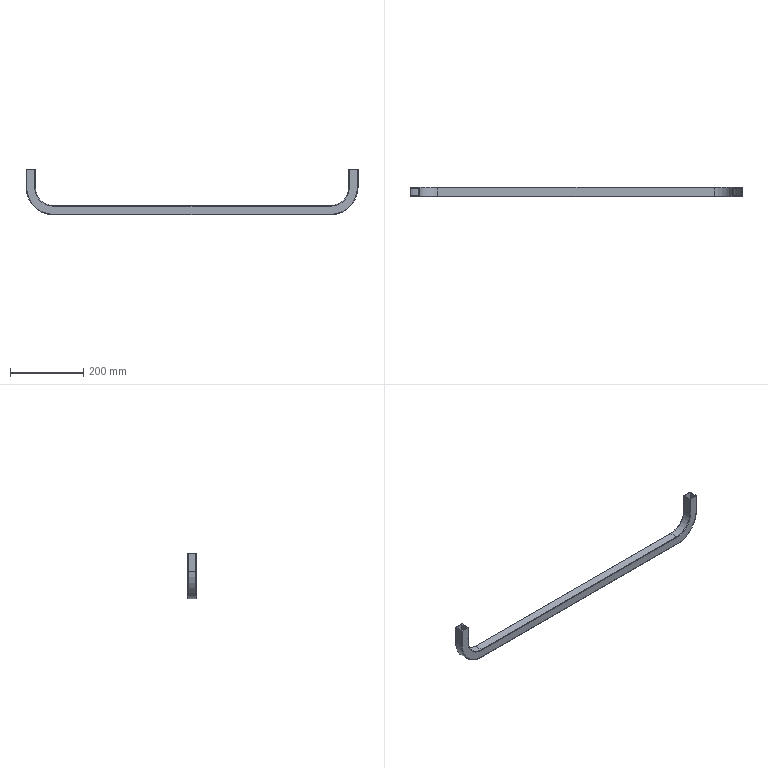Part | NX | features BREP 1 | 1 solid | 46 faces | box 908.05 x 25.4 x 125.476 mm | volume 193275 mm3 | cylinder 20 | plane 18 | torus 8 | commonest cylinder face diameters 3.175 x12 101.6 x2 105.562 x2 148.438 x2 152.4 x2
STEP:
#1=CARTESIAN_POINT('',(454.025,11.113,0.));
#2=VERTEX_POINT('',#1);
#3=CARTESIAN_POINT('',(452.438,12.7,0.));
#4=VERTEX_POINT('',#3);
#5=CARTESIAN_POINT('',(452.438,11.113,0.));
#6=DIRECTION('',(0.,0.,1.));
#7=DIRECTION('',(1.,0.,0.));
#8=AXIS2_PLACEMENT_3D('',#5,#6,#7);
#9=CIRCLE('',#8,1.588);
#10=EDGE_CURVE('',#2,#4,#9,.T.);
#11=ORIENTED_EDGE('',*,*,#10,.T.);
#12=CARTESIAN_POINT('',(430.212,12.7,0.));
#13=VERTEX_POINT('',#12);
#14=CARTESIAN_POINT('',(430.212,12.7,0.));
#15=DIRECTION('',(1.,0.,0.));
#16=VECTOR('',#15,1000.);
#17=LINE('',#14,#16);
#18=EDGE_CURVE('',#13,#4,#17,.T.);
#19=ORIENTED_EDGE('',*,*,#18,.F.);
#20=CARTESIAN_POINT('',(428.625,11.113,0.));
#21=VERTEX_POINT('',#20);
#22=CARTESIAN_POINT('',(430.212,11.113,0.));
#23=DIRECTION('',(0.,0.,1.));
#24=DIRECTION('',(0.,1.,0.));
#25=AXIS2_PLACEMENT_3D('',#22,#23,#24);
#26=CIRCLE('',#25,1.587);
#27=EDGE_CURVE('',#13,#21,#26,.T.);
#28=ORIENTED_EDGE('',*,*,#27,.T.);
#29=CARTESIAN_POINT('',(428.625,-11.113,0.));
#30=VERTEX_POINT('',#29);
#31=CARTESIAN_POINT('',(428.625,-11.113,0.));
#32=DIRECTION('',(0.,1.,0.));
#33=VECTOR('',#32,1000.);
#34=LINE('',#31,#33);
#35=EDGE_CURVE('',#30,#21,#34,.T.);
#36=ORIENTED_EDGE('',*,*,#35,.F.);
#37=CARTESIAN_POINT('',(430.212,-12.7,0.));
#38=VERTEX_POINT('',#37);
#39=CARTESIAN_POINT('',(430.212,-11.113,0.));
#40=DIRECTION('',(0.,0.,1.));
#41=DIRECTION('',(-1.,0.,0.));
#42=AXIS2_PLACEMENT_3D('',#39,#40,#41);
#43=CIRCLE('',#42,1.588);
#44=EDGE_CURVE('',#30,#38,#43,.T.);
#45=ORIENTED_EDGE('',*,*,#44,.T.);
#46=CARTESIAN_POINT('',(452.438,-12.7,0.));
#47=VERTEX_POINT('',#46);
#48=CARTESIAN_POINT('',(452.438,-12.7,0.));
#49=DIRECTION('',(-1.,0.,0.));
#50=VECTOR('',#49,1000.);
#51=LINE('',#48,#50);
#52=EDGE_CURVE('',#47,#38,#51,.T.);
#53=ORIENTED_EDGE('',*,*,#52,.F.);
#54=CARTESIAN_POINT('',(454.025,-11.113,0.));
#55=VERTEX_POINT('',#54);
#56=CARTESIAN_POINT('',(452.438,-11.113,0.));
#57=DIRECTION('',(0.,0.,1.));
#58=DIRECTION('',(0.,-1.,0.));
#59=AXIS2_PLACEMENT_3D('',#56,#57,#58);
#60=CIRCLE('',#59,1.587);
#61=EDGE_CURVE('',#47,#55,#60,.T.);
#62=ORIENTED_EDGE('',*,*,#61,.T.);
#63=CARTESIAN_POINT('',(454.025,11.113,0.));
#64=DIRECTION('',(0.,-1.,0.));
#65=VECTOR('',#64,1000.);
#66=LINE('',#63,#65);
#67=EDGE_CURVE('',#2,#55,#66,.T.);
#68=ORIENTED_EDGE('',*,*,#67,.F.);
#69=EDGE_LOOP('',(#11,#19,#28,#36,#45,#53,#62,#68));
#70=FACE_BOUND('',#69,.T.);
#71=CARTESIAN_POINT('',(452.044,-10.719,0.));
#72=VERTEX_POINT('',#71);
#73=CARTESIAN_POINT('',(452.044,10.719,0.));
#74=VERTEX_POINT('',#73);
#75=CARTESIAN_POINT('',(452.044,-10.719,0.));
#76=DIRECTION('',(0.,1.,0.));
#77=VECTOR('',#76,1000.);
#78=LINE('',#75,#77);
#79=EDGE_CURVE('',#72,#74,#78,.T.);
#80=ORIENTED_EDGE('',*,*,#79,.F.);
#81=CARTESIAN_POINT('',(430.606,-10.719,0.));
#82=VERTEX_POINT('',#81);
#83=CARTESIAN_POINT('',(430.606,-10.719,0.));
#84=DIRECTION('',(1.,0.,0.));
#85=VECTOR('',#84,1000.);
#86=LINE('',#83,#85);
#87=EDGE_CURVE('',#82,#72,#86,.T.);
#88=ORIENTED_EDGE('',*,*,#87,.F.);
#89=CARTESIAN_POINT('',(430.606,10.719,0.));
#90=VERTEX_POINT('',#89);
#91=CARTESIAN_POINT('',(430.606,10.719,0.));
#92=DIRECTION('',(0.,-1.,0.));
#93=VECTOR('',#92,1000.);
#94=LINE('',#91,#93);
#95=EDGE_CURVE('',#90,#82,#94,.T.);
#96=ORIENTED_EDGE('',*,*,#95,.F.);
#97=CARTESIAN_POINT('',(452.044,10.719,0.));
#98=DIRECTION('',(-1.,0.,0.));
#99=VECTOR('',#98,1000.);
#100=LINE('',#97,#99);
#101=EDGE_CURVE('',#74,#90,#100,.T.);
#102=ORIENTED_EDGE('',*,*,#101,.F.);
#103=EDGE_LOOP('',(#80,#88,#96,#102));
#104=FACE_BOUND('',#103,.T.);
#105=CARTESIAN_POINT('',(441.325,0.,0.));
#106=DIRECTION('',(0.,0.,-1.));
#107=DIRECTION('',(0.,-1.,0.));
#108=AXIS2_PLACEMENT_3D('',#105,#106,#107);
#109=PLANE('',#108);
#110=ADVANCED_FACE('',(#70,#104),#109,.F.);
#111=CARTESIAN_POINT('',(430.606,10.719,-49.276));
#112=VERTEX_POINT('',#111);
#113=CARTESIAN_POINT('',(430.606,10.719,0.));
#114=DIRECTION('',(0.,0.,-1.));
#115=VECTOR('',#114,1000.);
#116=LINE('',#113,#115);
#117=EDGE_CURVE('',#90,#112,#116,.T.);
#118=ORIENTED_EDGE('',*,*,#117,.T.);
#119=CARTESIAN_POINT('',(377.825,10.719,-102.057));
#120=VERTEX_POINT('',#119);
#121=CARTESIAN_POINT('',(377.825,10.719,-49.276));
#122=DIRECTION('',(0.,1.,0.));
#123=DIRECTION('',(1.,0.,0.));
#124=AXIS2_PLACEMENT_3D('',#121,#122,#123);
#125=CIRCLE('',#124,52.781);
#126=EDGE_CURVE('',#112,#120,#125,.T.);
#127=ORIENTED_EDGE('',*,*,#126,.T.);
#128=CARTESIAN_POINT('',(-377.825,10.719,-102.057));
#129=VERTEX_POINT('',#128);
#130=CARTESIAN_POINT('',(377.825,10.719,-102.057));
#131=DIRECTION('',(-1.,0.,0.));
#132=VECTOR('',#131,1000.);
#133=LINE('',#130,#132);
#134=EDGE_CURVE('',#120,#129,#133,.T.);
#135=ORIENTED_EDGE('',*,*,#134,.T.);
#136=CARTESIAN_POINT('',(-430.606,10.719,-49.276));
#137=VERTEX_POINT('',#136);
#138=CARTESIAN_POINT('',(-377.825,10.719,-49.276));
#139=DIRECTION('',(0.,1.,0.));
#140=DIRECTION('',(0.,0.,-1.));
#141=AXIS2_PLACEMENT_3D('',#138,#139,#140);
#142=CIRCLE('',#141,52.781);
#143=EDGE_CURVE('',#129,#137,#142,.T.);
#144=ORIENTED_EDGE('',*,*,#143,.T.);
#145=CARTESIAN_POINT('',(-430.606,10.719,0.));
#146=VERTEX_POINT('',#145);
#147=CARTESIAN_POINT('',(-430.606,10.719,-49.276));
#148=DIRECTION('',(0.,0.,1.));
#149=VECTOR('',#148,1000.);
#150=LINE('',#147,#149);
#151=EDGE_CURVE('',#137,#146,#150,.T.);
#152=ORIENTED_EDGE('',*,*,#151,.T.);
#153=CARTESIAN_POINT('',(-452.044,10.719,0.));
#154=VERTEX_POINT('',#153);
#155=CARTESIAN_POINT('',(-452.044,10.719,0.));
#156=DIRECTION('',(1.,0.,0.));
#157=VECTOR('',#156,1000.);
#158=LINE('',#155,#157);
#159=EDGE_CURVE('',#154,#146,#158,.T.);
#160=ORIENTED_EDGE('',*,*,#159,.F.);
#161=CARTESIAN_POINT('',(-452.044,10.719,-49.276));
#162=VERTEX_POINT('',#161);
#163=CARTESIAN_POINT('',(-452.044,10.719,-49.276));
#164=DIRECTION('',(0.,0.,1.));
#165=VECTOR('',#164,1000.);
#166=LINE('',#163,#165);
#167=EDGE_CURVE('',#162,#154,#166,.T.);
#168=ORIENTED_EDGE('',*,*,#167,.F.);
#169=CARTESIAN_POINT('',(-377.825,10.719,-123.495));
#170=VERTEX_POINT('',#169);
#171=CARTESIAN_POINT('',(-377.825,10.719,-49.276));
#172=DIRECTION('',(0.,1.,0.));
#173=DIRECTION('',(0.,0.,-1.));
#174=AXIS2_PLACEMENT_3D('',#171,#172,#173);
#175=CIRCLE('',#174,74.219);
#176=EDGE_CURVE('',#170,#162,#175,.T.);
#177=ORIENTED_EDGE('',*,*,#176,.F.);
#178=CARTESIAN_POINT('',(377.825,10.719,-123.495));
#179=VERTEX_POINT('',#178);
#180=CARTESIAN_POINT('',(377.825,10.719,-123.495));
#181=DIRECTION('',(-1.,0.,0.));
#182=VECTOR('',#181,1000.);
#183=LINE('',#180,#182);
#184=EDGE_CURVE('',#179,#170,#183,.T.);
#185=ORIENTED_EDGE('',*,*,#184,.F.);
#186=CARTESIAN_POINT('',(452.044,10.719,-49.276));
#187=VERTEX_POINT('',#186);
#188=CARTESIAN_POINT('',(377.825,10.719,-49.276));
#189=DIRECTION('',(0.,1.,0.));
#190=DIRECTION('',(1.,0.,0.));
#191=AXIS2_PLACEMENT_3D('',#188,#189,#190);
#192=CIRCLE('',#191,74.219);
#193=EDGE_CURVE('',#187,#179,#192,.T.);
#194=ORIENTED_EDGE('',*,*,#193,.F.);
#195=CARTESIAN_POINT('',(452.044,10.719,0.));
#196=DIRECTION('',(0.,0.,-1.));
#197=VECTOR('',#196,1000.);
#198=LINE('',#195,#197);
#199=EDGE_CURVE('',#74,#187,#198,.T.);
#200=ORIENTED_EDGE('',*,*,#199,.F.);
#201=ORIENTED_EDGE('',*,*,#101,.T.);
#202=EDGE_LOOP('',(#118,#127,#135,#144,#152,#160,#168,#177,#185,#194,#200,#201));
#203=FACE_BOUND('',#202,.T.);
#204=CARTESIAN_POINT('',(452.044,10.719,0.));
#205=DIRECTION('',(0.,-1.,0.));
#206=DIRECTION('',(0.,0.,-1.));
#207=AXIS2_PLACEMENT_3D('',#204,#205,#206);
#208=PLANE('',#207);
#209=ADVANCED_FACE('',(#203),#208,.T.);
#210=ORIENTED_EDGE('',*,*,#199,.T.);
#211=CARTESIAN_POINT('',(452.044,-10.719,-49.276));
#212=VERTEX_POINT('',#211);
#213=CARTESIAN_POINT('',(452.044,-10.719,-49.276));
#214=DIRECTION('',(0.,1.,0.));
#215=VECTOR('',#214,1000.);
#216=LINE('',#213,#215);
#217=EDGE_CURVE('',#212,#187,#216,.T.);
#218=ORIENTED_EDGE('',*,*,#217,.F.);
#219=CARTESIAN_POINT('',(452.044,-10.719,0.));
#220=DIRECTION('',(0.,0.,-1.));
#221=VECTOR('',#220,1000.);
#222=LINE('',#219,#221);
#223=EDGE_CURVE('',#72,#212,#222,.T.);
#224=ORIENTED_EDGE('',*,*,#223,.F.);
#225=ORIENTED_EDGE('',*,*,#79,.T.);
#226=EDGE_LOOP('',(#210,#218,#224,#225));
#227=FACE_BOUND('',#226,.T.);
#228=CARTESIAN_POINT('',(452.044,-10.719,0.));
#229=DIRECTION('',(-1.,0.,0.));
#230=DIRECTION('',(0.,0.,1.));
#231=AXIS2_PLACEMENT_3D('',#228,#229,#230);
#232=PLANE('',#231);
#233=ADVANCED_FACE('',(#227),#232,.T.);
#234=ORIENTED_EDGE('',*,*,#223,.T.);
#235=CARTESIAN_POINT('',(377.825,-10.719,-123.495));
#236=VERTEX_POINT('',#235);
#237=CARTESIAN_POINT('',(377.825,-10.719,-49.276));
#238=DIRECTION('',(0.,1.,0.));
#239=DIRECTION('',(1.,0.,0.));
#240=AXIS2_PLACEMENT_3D('',#237,#238,#239);
#241=CIRCLE('',#240,74.219);
#242=EDGE_CURVE('',#212,#236,#241,.T.);
#243=ORIENTED_EDGE('',*,*,#242,.T.);
#244=CARTESIAN_POINT('',(-377.825,-10.719,-123.495));
#245=VERTEX_POINT('',#244);
#246=CARTESIAN_POINT('',(377.825,-10.719,-123.495));
#247=DIRECTION('',(-1.,0.,0.));
#248=VECTOR('',#247,1000.);
#249=LINE('',#246,#248);
#250=EDGE_CURVE('',#236,#245,#249,.T.);
#251=ORIENTED_EDGE('',*,*,#250,.T.);
#252=CARTESIAN_POINT('',(-452.044,-10.719,-49.276));
#253=VERTEX_POINT('',#252);
#254=CARTESIAN_POINT('',(-377.825,-10.719,-49.276));
#255=DIRECTION('',(0.,1.,0.));
#256=DIRECTION('',(0.,0.,-1.));
#257=AXIS2_PLACEMENT_3D('',#254,#255,#256);
#258=CIRCLE('',#257,74.219);
#259=EDGE_CURVE('',#245,#253,#258,.T.);
#260=ORIENTED_EDGE('',*,*,#259,.T.);
#261=CARTESIAN_POINT('',(-452.044,-10.719,0.));
#262=VERTEX_POINT('',#261);
#263=CARTESIAN_POINT('',(-452.044,-10.719,-49.276));
#264=DIRECTION('',(0.,0.,1.));
#265=VECTOR('',#264,1000.);
#266=LINE('',#263,#265);
#267=EDGE_CURVE('',#253,#262,#266,.T.);
#268=ORIENTED_EDGE('',*,*,#267,.T.);
#269=CARTESIAN_POINT('',(-430.606,-10.719,0.));
#270=VERTEX_POINT('',#269);
#271=CARTESIAN_POINT('',(-430.606,-10.719,0.));
#272=DIRECTION('',(-1.,0.,0.));
#273=VECTOR('',#272,1000.);
#274=LINE('',#271,#273);
#275=EDGE_CURVE('',#270,#262,#274,.T.);
#276=ORIENTED_EDGE('',*,*,#275,.F.);
#277=CARTESIAN_POINT('',(-430.606,-10.719,-49.276));
#278=VERTEX_POINT('',#277);
#279=CARTESIAN_POINT('',(-430.606,-10.719,-49.276));
#280=DIRECTION('',(0.,0.,1.));
#281=VECTOR('',#280,1000.);
#282=LINE('',#279,#281);
#283=EDGE_CURVE('',#278,#270,#282,.T.);
#284=ORIENTED_EDGE('',*,*,#283,.F.);
#285=CARTESIAN_POINT('',(-377.825,-10.719,-102.057));
#286=VERTEX_POINT('',#285);
#287=CARTESIAN_POINT('',(-377.825,-10.719,-49.276));
#288=DIRECTION('',(0.,1.,0.));
#289=DIRECTION('',(0.,0.,-1.));
#290=AXIS2_PLACEMENT_3D('',#287,#288,#289);
#291=CIRCLE('',#290,52.781);
#292=EDGE_CURVE('',#286,#278,#291,.T.);
#293=ORIENTED_EDGE('',*,*,#292,.F.);
#294=CARTESIAN_POINT('',(377.825,-10.719,-102.057));
#295=VERTEX_POINT('',#294);
#296=CARTESIAN_POINT('',(377.825,-10.719,-102.057));
#297=DIRECTION('',(-1.,0.,0.));
#298=VECTOR('',#297,1000.);
#299=LINE('',#296,#298);
#300=EDGE_CURVE('',#295,#286,#299,.T.);
#301=ORIENTED_EDGE('',*,*,#300,.F.);
#302=CARTESIAN_POINT('',(430.606,-10.719,-49.276));
#303=VERTEX_POINT('',#302);
#304=CARTESIAN_POINT('',(377.825,-10.719,-49.276));
#305=DIRECTION('',(0.,1.,0.));
#306=DIRECTION('',(1.,0.,0.));
#307=AXIS2_PLACEMENT_3D('',#304,#305,#306);
#308=CIRCLE('',#307,52.781);
#309=EDGE_CURVE('',#303,#295,#308,.T.);
#310=ORIENTED_EDGE('',*,*,#309,.F.);
#311=CARTESIAN_POINT('',(430.606,-10.719,0.));
#312=DIRECTION('',(0.,0.,-1.));
#313=VECTOR('',#312,1000.);
#314=LINE('',#311,#313);
#315=EDGE_CURVE('',#82,#303,#314,.T.);
#316=ORIENTED_EDGE('',*,*,#315,.F.);
#317=ORIENTED_EDGE('',*,*,#87,.T.);
#318=EDGE_LOOP('',(#234,#243,#251,#260,#268,#276,#284,#293,#301,#310,#316,#317));
#319=FACE_BOUND('',#318,.T.);
#320=CARTESIAN_POINT('',(430.606,-10.719,0.));
#321=DIRECTION('',(0.,1.,0.));
#322=DIRECTION('',(1.,0.,0.));
#323=AXIS2_PLACEMENT_3D('',#320,#321,#322);
#324=PLANE('',#323);
#325=ADVANCED_FACE('',(#319),#324,.T.);
#326=ORIENTED_EDGE('',*,*,#315,.T.);
#327=CARTESIAN_POINT('',(430.606,10.719,-49.276));
#328=DIRECTION('',(0.,-1.,0.));
#329=VECTOR('',#328,1000.);
#330=LINE('',#327,#329);
#331=EDGE_CURVE('',#112,#303,#330,.T.);
#332=ORIENTED_EDGE('',*,*,#331,.F.);
#333=ORIENTED_EDGE('',*,*,#117,.F.);
#334=ORIENTED_EDGE('',*,*,#95,.T.);
#335=EDGE_LOOP('',(#326,#332,#333,#334));
#336=FACE_BOUND('',#335,.T.);
#337=CARTESIAN_POINT('',(430.606,10.719,0.));
#338=DIRECTION('',(1.,0.,0.));
#339=DIRECTION('',(0.,1.,0.));
#340=AXIS2_PLACEMENT_3D('',#337,#338,#339);
#341=PLANE('',#340);
#342=ADVANCED_FACE('',(#336),#341,.T.);
#343=ORIENTED_EDGE('',*,*,#309,.T.);
#344=CARTESIAN_POINT('',(377.825,10.719,-102.057));
#345=DIRECTION('',(0.,-1.,0.));
#346=VECTOR('',#345,1000.);
#347=LINE('',#344,#346);
#348=EDGE_CURVE('',#120,#295,#347,.T.);
#349=ORIENTED_EDGE('',*,*,#348,.F.);
#350=ORIENTED_EDGE('',*,*,#126,.F.);
#351=ORIENTED_EDGE('',*,*,#331,.T.);
#352=EDGE_LOOP('',(#343,#349,#350,#351));
#353=FACE_BOUND('',#352,.T.);
#354=CARTESIAN_POINT('',(377.825,-25.4,-49.276));
#355=DIRECTION('',(0.,1.,0.));
#356=DIRECTION('',(-1.,0.,0.));
#357=AXIS2_PLACEMENT_3D('',#354,#355,#356);
#358=CYLINDRICAL_SURFACE('',#357,52.781);
#359=ADVANCED_FACE('',(#353),#358,.T.);
#360=ORIENTED_EDGE('',*,*,#300,.T.);
#361=CARTESIAN_POINT('',(-377.825,10.719,-102.057));
#362=DIRECTION('',(0.,-1.,0.));
#363=VECTOR('',#362,1000.);
#364=LINE('',#361,#363);
#365=EDGE_CURVE('',#129,#286,#364,.T.);
#366=ORIENTED_EDGE('',*,*,#365,.F.);
#367=ORIENTED_EDGE('',*,*,#134,.F.);
#368=ORIENTED_EDGE('',*,*,#348,.T.);
#369=EDGE_LOOP('',(#360,#366,#367,#368));
#370=FACE_BOUND('',#369,.T.);
#371=CARTESIAN_POINT('',(377.825,10.719,-102.057));
#372=DIRECTION('',(0.,0.,-1.));
#373=DIRECTION('',(0.,-1.,0.));
#374=AXIS2_PLACEMENT_3D('',#371,#372,#373);
#375=PLANE('',#374);
#376=ADVANCED_FACE('',(#370),#375,.T.);
#377=ORIENTED_EDGE('',*,*,#292,.T.);
#378=CARTESIAN_POINT('',(-430.606,10.719,-49.276));
#379=DIRECTION('',(0.,-1.,0.));
#380=VECTOR('',#379,1000.);
#381=LINE('',#378,#380);
#382=EDGE_CURVE('',#137,#278,#381,.T.);
#383=ORIENTED_EDGE('',*,*,#382,.F.);
#384=ORIENTED_EDGE('',*,*,#143,.F.);
#385=ORIENTED_EDGE('',*,*,#365,.T.);
#386=EDGE_LOOP('',(#377,#383,#384,#385));
#387=FACE_BOUND('',#386,.T.);
#388=CARTESIAN_POINT('',(-377.825,-25.4,-49.276));
#389=DIRECTION('',(0.,1.,0.));
#390=DIRECTION('',(0.,0.,1.));
#391=AXIS2_PLACEMENT_3D('',#388,#389,#390);
#392=CYLINDRICAL_SURFACE('',#391,52.781);
#393=ADVANCED_FACE('',(#387),#392,.T.);
#394=ORIENTED_EDGE('',*,*,#283,.T.);
#395=CARTESIAN_POINT('',(-430.606,10.719,0.));
#396=DIRECTION('',(0.,-1.,0.));
#397=VECTOR('',#396,1000.);
#398=LINE('',#395,#397);
#399=EDGE_CURVE('',#146,#270,#398,.T.);
#400=ORIENTED_EDGE('',*,*,#399,.F.);
#401=ORIENTED_EDGE('',*,*,#151,.F.);
#402=ORIENTED_EDGE('',*,*,#382,.T.);
#403=EDGE_LOOP('',(#394,#400,#401,#402));
#404=FACE_BOUND('',#403,.T.);
#405=CARTESIAN_POINT('',(-430.606,10.719,-49.276));
#406=DIRECTION('',(-1.,0.,0.));
#407=DIRECTION('',(0.,0.,1.));
#408=AXIS2_PLACEMENT_3D('',#405,#406,#407);
#409=PLANE('',#408);
#410=ADVANCED_FACE('',(#404),#409,.T.);
#411=CARTESIAN_POINT('',(-454.025,-11.113,0.));
#412=VERTEX_POINT('',#411);
#413=CARTESIAN_POINT('',(-452.438,-12.7,0.));
#414=VERTEX_POINT('',#413);
#415=CARTESIAN_POINT('',(-452.438,-11.113,0.));
#416=DIRECTION('',(0.,0.,1.));
#417=DIRECTION('',(-1.,0.,0.));
#418=AXIS2_PLACEMENT_3D('',#415,#416,#417);
#419=CIRCLE('',#418,1.588);
#420=EDGE_CURVE('',#412,#414,#419,.T.);
#421=ORIENTED_EDGE('',*,*,#420,.T.);
#422=CARTESIAN_POINT('',(-430.212,-12.7,0.));
#423=VERTEX_POINT('',#422);
#424=CARTESIAN_POINT('',(-452.438,-12.7,0.));
#425=DIRECTION('',(1.,0.,0.));
#426=VECTOR('',#425,1000.);
#427=LINE('',#424,#426);
#428=EDGE_CURVE('',#414,#423,#427,.T.);
#429=ORIENTED_EDGE('',*,*,#428,.T.);
#430=CARTESIAN_POINT('',(-428.625,-11.113,0.));
#431=VERTEX_POINT('',#430);
#432=CARTESIAN_POINT('',(-430.212,-11.113,0.));
#433=DIRECTION('',(0.,0.,1.));
#434=DIRECTION('',(0.,-1.,0.));
#435=AXIS2_PLACEMENT_3D('',#432,#433,#434);
#436=CIRCLE('',#435,1.587);
#437=EDGE_CURVE('',#423,#431,#436,.T.);
#438=ORIENTED_EDGE('',*,*,#437,.T.);
#439=CARTESIAN_POINT('',(-428.625,11.113,0.));
#440=VERTEX_POINT('',#439);
#441=CARTESIAN_POINT('',(-428.625,-11.113,0.));
#442=DIRECTION('',(0.,1.,0.));
#443=VECTOR('',#442,1000.);
#444=LINE('',#441,#443);
#445=EDGE_CURVE('',#431,#440,#444,.T.);
#446=ORIENTED_EDGE('',*,*,#445,.T.);
#447=CARTESIAN_POINT('',(-430.212,12.7,0.));
#448=VERTEX_POINT('',#447);
#449=CARTESIAN_POINT('',(-430.212,11.113,0.));
#450=DIRECTION('',(0.,0.,1.));
#451=DIRECTION('',(1.,0.,0.));
#452=AXIS2_PLACEMENT_3D('',#449,#450,#451);
#453=CIRCLE('',#452,1.588);
#454=EDGE_CURVE('',#440,#448,#453,.T.);
#455=ORIENTED_EDGE('',*,*,#454,.T.);
#456=CARTESIAN_POINT('',(-452.438,12.7,0.));
#457=VERTEX_POINT('',#456);
#458=CARTESIAN_POINT('',(-430.212,12.7,0.));
#459=DIRECTION('',(-1.,0.,0.));
#460=VECTOR('',#459,1000.);
#461=LINE('',#458,#460);
#462=EDGE_CURVE('',#448,#457,#461,.T.);
#463=ORIENTED_EDGE('',*,*,#462,.T.);
#464=CARTESIAN_POINT('',(-454.025,11.113,0.));
#465=VERTEX_POINT('',#464);
#466=CARTESIAN_POINT('',(-452.438,11.113,0.));
#467=DIRECTION('',(0.,0.,1.));
#468=DIRECTION('',(0.,1.,0.));
#469=AXIS2_PLACEMENT_3D('',#466,#467,#468);
#470=CIRCLE('',#469,1.587);
#471=EDGE_CURVE('',#457,#465,#470,.T.);
#472=ORIENTED_EDGE('',*,*,#471,.T.);
#473=CARTESIAN_POINT('',(-454.025,11.113,0.));
#474=DIRECTION('',(0.,-1.,0.));
#475=VECTOR('',#474,1000.);
#476=LINE('',#473,#475);
#477=EDGE_CURVE('',#465,#412,#476,.T.);
#478=ORIENTED_EDGE('',*,*,#477,.T.);
#479=EDGE_LOOP('',(#421,#429,#438,#446,#455,#463,#472,#478));
#480=FACE_BOUND('',#479,.T.);
#481=ORIENTED_EDGE('',*,*,#399,.T.);
#482=ORIENTED_EDGE('',*,*,#275,.T.);
#483=CARTESIAN_POINT('',(-452.044,-10.719,0.));
#484=DIRECTION('',(0.,1.,0.));
#485=VECTOR('',#484,1000.);
#486=LINE('',#483,#485);
#487=EDGE_CURVE('',#262,#154,#486,.T.);
#488=ORIENTED_EDGE('',*,*,#487,.T.);
#489=ORIENTED_EDGE('',*,*,#159,.T.);
#490=EDGE_LOOP('',(#481,#482,#488,#489));
#491=FACE_BOUND('',#490,.T.);
#492=CARTESIAN_POINT('',(-441.325,0.,0.));
#493=DIRECTION('',(0.,0.,1.));
#494=DIRECTION('',(1.,0.,0.));
#495=AXIS2_PLACEMENT_3D('',#492,#493,#494);
#496=PLANE('',#495);
#497=ADVANCED_FACE('',(#480,#491),#496,.T.);
#498=ORIENTED_EDGE('',*,*,#167,.T.);
#499=ORIENTED_EDGE('',*,*,#487,.F.);
#500=ORIENTED_EDGE('',*,*,#267,.F.);
#501=CARTESIAN_POINT('',(-452.044,-10.719,-49.276));
#502=DIRECTION('',(0.,1.,0.));
#503=VECTOR('',#502,1000.);
#504=LINE('',#501,#503);
#505=EDGE_CURVE('',#253,#162,#504,.T.);
#506=ORIENTED_EDGE('',*,*,#505,.T.);
#507=EDGE_LOOP('',(#498,#499,#500,#506));
#508=FACE_BOUND('',#507,.T.);
#509=CARTESIAN_POINT('',(-452.044,-10.719,-49.276));
#510=DIRECTION('',(1.,0.,0.));
#511=DIRECTION('',(0.,1.,0.));
#512=AXIS2_PLACEMENT_3D('',#509,#510,#511);
#513=PLANE('',#512);
#514=ADVANCED_FACE('',(#508),#513,.T.);
#515=ORIENTED_EDGE('',*,*,#176,.T.);
#516=ORIENTED_EDGE('',*,*,#505,.F.);
#517=ORIENTED_EDGE('',*,*,#259,.F.);
#518=CARTESIAN_POINT('',(-377.825,-10.719,-123.495));
#519=DIRECTION('',(0.,1.,0.));
#520=VECTOR('',#519,1000.);
#521=LINE('',#518,#520);
#522=EDGE_CURVE('',#245,#170,#521,.T.);
#523=ORIENTED_EDGE('',*,*,#522,.T.);
#524=EDGE_LOOP('',(#515,#516,#517,#523));
#525=FACE_BOUND('',#524,.T.);
#526=CARTESIAN_POINT('',(-377.825,-25.4,-49.276));
#527=DIRECTION('',(0.,1.,0.));
#528=DIRECTION('',(0.,0.,1.));
#529=AXIS2_PLACEMENT_3D('',#526,#527,#528);
#530=CYLINDRICAL_SURFACE('',#529,74.219);
#531=ADVANCED_FACE('',(#525),#530,.F.);
#532=ORIENTED_EDGE('',*,*,#184,.T.);
#533=ORIENTED_EDGE('',*,*,#522,.F.);
#534=ORIENTED_EDGE('',*,*,#250,.F.);
#535=CARTESIAN_POINT('',(377.825,-10.719,-123.495));
#536=DIRECTION('',(0.,1.,0.));
#537=VECTOR('',#536,1000.);
#538=LINE('',#535,#537);
#539=EDGE_CURVE('',#236,#179,#538,.T.);
#540=ORIENTED_EDGE('',*,*,#539,.T.);
#541=EDGE_LOOP('',(#532,#533,#534,#540));
#542=FACE_BOUND('',#541,.T.);
#543=CARTESIAN_POINT('',(377.825,-10.719,-123.495));
#544=DIRECTION('',(0.,0.,1.));
#545=DIRECTION('',(1.,0.,0.));
#546=AXIS2_PLACEMENT_3D('',#543,#544,#545);
#547=PLANE('',#546);
#548=ADVANCED_FACE('',(#542),#547,.T.);
#549=ORIENTED_EDGE('',*,*,#193,.T.);
#550=ORIENTED_EDGE('',*,*,#539,.F.);
#551=ORIENTED_EDGE('',*,*,#242,.F.);
#552=ORIENTED_EDGE('',*,*,#217,.T.);
#553=EDGE_LOOP('',(#549,#550,#551,#552));
#554=FACE_BOUND('',#553,.T.);
#555=CARTESIAN_POINT('',(377.825,-25.4,-49.276));
#556=DIRECTION('',(0.,1.,0.));
#557=DIRECTION('',(-1.,0.,0.));
#558=AXIS2_PLACEMENT_3D('',#555,#556,#557);
#559=CYLINDRICAL_SURFACE('',#558,74.219);
#560=ADVANCED_FACE('',(#554),#559,.F.);
#561=CARTESIAN_POINT('',(-454.025,-11.113,-49.276));
#562=VERTEX_POINT('',#561);
#563=CARTESIAN_POINT('',(-454.025,-11.113,0.));
#564=DIRECTION('',(0.,0.,-1.));
#565=VECTOR('',#564,1000.);
#566=LINE('',#563,#565);
#567=EDGE_CURVE('',#412,#562,#566,.T.);
#568=ORIENTED_EDGE('',*,*,#567,.F.);
#569=ORIENTED_EDGE('',*,*,#477,.F.);
#570=CARTESIAN_POINT('',(-454.025,11.113,-49.276));
#571=VERTEX_POINT('',#570);
#572=CARTESIAN_POINT('',(-454.025,11.113,0.));
#573=DIRECTION('',(0.,0.,-1.));
#574=VECTOR('',#573,1000.);
#575=LINE('',#572,#574);
#576=EDGE_CURVE('',#465,#571,#575,.T.);
#577=ORIENTED_EDGE('',*,*,#576,.T.);
#578=CARTESIAN_POINT('',(-454.025,11.113,-49.276));
#579=DIRECTION('',(0.,-1.,0.));
#580=VECTOR('',#579,1000.);
#581=LINE('',#578,#580);
#582=EDGE_CURVE('',#571,#562,#581,.T.);
#583=ORIENTED_EDGE('',*,*,#582,.T.);
#584=EDGE_LOOP('',(#568,#569,#577,#583));
#585=FACE_BOUND('',#584,.T.);
#586=CARTESIAN_POINT('',(-454.025,12.7,-49.276));
#587=DIRECTION('',(-1.,0.,0.));
#588=DIRECTION('',(0.,0.,1.));
#589=AXIS2_PLACEMENT_3D('',#586,#587,#588);
#590=PLANE('',#589);
#591=ADVANCED_FACE('',(#585),#590,.T.);
#592=CARTESIAN_POINT('',(-377.825,11.113,-125.476));
#593=VERTEX_POINT('',#592);
#594=CARTESIAN_POINT('',(-377.825,11.113,-49.276));
#595=DIRECTION('',(0.,-1.,0.));
#596=DIRECTION('',(-1.,0.,0.));
#597=AXIS2_PLACEMENT_3D('',#594,#595,#596);
#598=CIRCLE('',#597,76.2);
#599=EDGE_CURVE('',#571,#593,#598,.T.);
#600=ORIENTED_EDGE('',*,*,#599,.T.);
#601=CARTESIAN_POINT('',(-377.825,-11.113,-125.476));
#602=VERTEX_POINT('',#601);
#603=CARTESIAN_POINT('',(-377.825,11.113,-125.476));
#604=DIRECTION('',(0.,-1.,0.));
#605=VECTOR('',#604,1000.);
#606=LINE('',#603,#605);
#607=EDGE_CURVE('',#593,#602,#606,.T.);
#608=ORIENTED_EDGE('',*,*,#607,.T.);
#609=CARTESIAN_POINT('',(-377.825,-11.113,-49.276));
#610=DIRECTION('',(0.,-1.,0.));
#611=DIRECTION('',(-1.,0.,0.));
#612=AXIS2_PLACEMENT_3D('',#609,#610,#611);
#613=CIRCLE('',#612,76.2);
#614=EDGE_CURVE('',#562,#602,#613,.T.);
#615=ORIENTED_EDGE('',*,*,#614,.F.);
#616=ORIENTED_EDGE('',*,*,#582,.F.);
#617=EDGE_LOOP('',(#600,#608,#615,#616));
#618=FACE_BOUND('',#617,.T.);
#619=CARTESIAN_POINT('',(-377.825,-25.4,-49.276));
#620=DIRECTION('',(0.,1.,0.));
#621=DIRECTION('',(0.,0.,1.));
#622=AXIS2_PLACEMENT_3D('',#619,#620,#621);
#623=CYLINDRICAL_SURFACE('',#622,76.2);
#624=ADVANCED_FACE('',(#618),#623,.T.);
#625=CARTESIAN_POINT('',(-452.438,-12.7,-49.276));
#626=VERTEX_POINT('',#625);
#627=CARTESIAN_POINT('',(-452.438,-11.113,-49.276));
#628=DIRECTION('',(0.,0.,-1.));
#629=DIRECTION('',(0.,-1.,0.));
#630=AXIS2_PLACEMENT_3D('',#627,#628,#629);
#631=CIRCLE('',#630,1.587);
#632=EDGE_CURVE('',#626,#562,#631,.T.);
#633=ORIENTED_EDGE('',*,*,#632,.T.);
#634=ORIENTED_EDGE('',*,*,#614,.T.);
#635=CARTESIAN_POINT('',(-377.825,-12.7,-123.888));
#636=VERTEX_POINT('',#635);
#637=CARTESIAN_POINT('',(-377.825,-11.113,-123.888));
#638=DIRECTION('',(1.,0.,0.));
#639=DIRECTION('',(0.,-1.,0.));
#640=AXIS2_PLACEMENT_3D('',#637,#638,#639);
#641=CIRCLE('',#640,1.587);
#642=EDGE_CURVE('',#636,#602,#641,.T.);
#643=ORIENTED_EDGE('',*,*,#642,.F.);
#644=CARTESIAN_POINT('',(-377.825,-12.7,-49.276));
#645=DIRECTION('',(0.,-1.,0.));
#646=DIRECTION('',(-1.,0.,0.));
#647=AXIS2_PLACEMENT_3D('',#644,#645,#646);
#648=CIRCLE('',#647,74.613);
#649=EDGE_CURVE('',#626,#636,#648,.T.);
#650=ORIENTED_EDGE('',*,*,#649,.F.);
#651=EDGE_LOOP('',(#633,#634,#643,#650));
#652=FACE_BOUND('',#651,.T.);
#653=CARTESIAN_POINT('',(-377.825,-11.113,-49.276));
#654=DIRECTION('',(0.,1.,0.));
#655=DIRECTION('',(-0.9997,0.,0.02628));
#656=AXIS2_PLACEMENT_3D('',#653,#654,#655);
#657=TOROIDAL_SURFACE('',#656,74.612,1.587);
#658=ADVANCED_FACE('',(#652),#657,.T.);
#659=CARTESIAN_POINT('',(430.212,-12.7,-49.276));
#660=VERTEX_POINT('',#659);
#661=CARTESIAN_POINT('',(430.212,-12.7,-49.276));
#662=DIRECTION('',(0.,0.,1.));
#663=VECTOR('',#662,1000.);
#664=LINE('',#661,#663);
#665=EDGE_CURVE('',#660,#38,#664,.T.);
#666=ORIENTED_EDGE('',*,*,#665,.F.);
#667=CARTESIAN_POINT('',(377.825,-12.7,-101.664));
#668=VERTEX_POINT('',#667);
#669=CARTESIAN_POINT('',(377.825,-12.7,-49.276));
#670=DIRECTION('',(0.,-1.,0.));
#671=DIRECTION('',(0.,0.,-1.));
#672=AXIS2_PLACEMENT_3D('',#669,#670,#671);
#673=CIRCLE('',#672,52.388);
#674=EDGE_CURVE('',#668,#660,#673,.T.);
#675=ORIENTED_EDGE('',*,*,#674,.F.);
#676=CARTESIAN_POINT('',(-377.825,-12.7,-101.663));
#677=VERTEX_POINT('',#676);
#678=CARTESIAN_POINT('',(-377.825,-12.7,-101.663));
#679=DIRECTION('',(1.,0.,0.));
#680=VECTOR('',#679,1000.);
#681=LINE('',#678,#680);
#682=EDGE_CURVE('',#677,#668,#681,.T.);
#683=ORIENTED_EDGE('',*,*,#682,.F.);
#684=CARTESIAN_POINT('',(-430.213,-12.7,-49.276));
#685=VERTEX_POINT('',#684);
#686=CARTESIAN_POINT('',(-377.825,-12.7,-49.276));
#687=DIRECTION('',(0.,-1.,0.));
#688=DIRECTION('',(-1.,0.,0.));
#689=AXIS2_PLACEMENT_3D('',#686,#687,#688);
#690=CIRCLE('',#689,52.388);
#691=EDGE_CURVE('',#685,#677,#690,.T.);
#692=ORIENTED_EDGE('',*,*,#691,.F.);
#693=CARTESIAN_POINT('',(-430.212,-12.7,0.));
#694=DIRECTION('',(0.,0.,-1.));
#695=VECTOR('',#694,1000.);
#696=LINE('',#693,#695);
#697=EDGE_CURVE('',#423,#685,#696,.T.);
#698=ORIENTED_EDGE('',*,*,#697,.F.);
#699=ORIENTED_EDGE('',*,*,#428,.F.);
#700=CARTESIAN_POINT('',(-452.438,-12.7,0.));
#701=DIRECTION('',(0.,0.,-1.));
#702=VECTOR('',#701,1000.);
#703=LINE('',#700,#702);
#704=EDGE_CURVE('',#414,#626,#703,.T.);
#705=ORIENTED_EDGE('',*,*,#704,.T.);
#706=ORIENTED_EDGE('',*,*,#649,.T.);
#707=CARTESIAN_POINT('',(377.825,-12.7,-123.889));
#708=VERTEX_POINT('',#707);
#709=CARTESIAN_POINT('',(-377.825,-12.7,-123.888));
#710=DIRECTION('',(1.,0.,0.));
#711=VECTOR('',#710,1000.);
#712=LINE('',#709,#711);
#713=EDGE_CURVE('',#636,#708,#712,.T.);
#714=ORIENTED_EDGE('',*,*,#713,.T.);
#715=CARTESIAN_POINT('',(452.438,-12.7,-49.276));
#716=VERTEX_POINT('',#715);
#717=CARTESIAN_POINT('',(377.825,-12.7,-49.276));
#718=DIRECTION('',(0.,-1.,0.));
#719=DIRECTION('',(0.,0.,-1.));
#720=AXIS2_PLACEMENT_3D('',#717,#718,#719);
#721=CIRCLE('',#720,74.613);
#722=EDGE_CURVE('',#708,#716,#721,.T.);
#723=ORIENTED_EDGE('',*,*,#722,.T.);
#724=CARTESIAN_POINT('',(452.438,-12.7,-49.276));
#725=DIRECTION('',(0.,0.,1.));
#726=VECTOR('',#725,1000.);
#727=LINE('',#724,#726);
#728=EDGE_CURVE('',#716,#47,#727,.T.);
#729=ORIENTED_EDGE('',*,*,#728,.T.);
#730=ORIENTED_EDGE('',*,*,#52,.T.);
#731=EDGE_LOOP('',(#666,#675,#683,#692,#698,#699,#705,#706,#714,#723,#729,#730));
#732=FACE_BOUND('',#731,.T.);
#733=CARTESIAN_POINT('',(454.025,-12.7,0.));
#734=DIRECTION('',(0.,-1.,0.));
#735=DIRECTION('',(0.,0.,-1.));
#736=AXIS2_PLACEMENT_3D('',#733,#734,#735);
#737=PLANE('',#736);
#738=ADVANCED_FACE('',(#732),#737,.T.);
#739=CARTESIAN_POINT('',(454.025,-11.113,-49.276));
#740=VERTEX_POINT('',#739);
#741=CARTESIAN_POINT('',(452.438,-11.113,-49.276));
#742=DIRECTION('',(0.,0.,1.));
#743=DIRECTION('',(0.,-1.,0.));
#744=AXIS2_PLACEMENT_3D('',#741,#742,#743);
#745=CIRCLE('',#744,1.587);
#746=EDGE_CURVE('',#716,#740,#745,.T.);
#747=ORIENTED_EDGE('',*,*,#746,.T.);
#748=CARTESIAN_POINT('',(454.025,-11.113,-49.276));
#749=DIRECTION('',(0.,0.,1.));
#750=VECTOR('',#749,1000.);
#751=LINE('',#748,#750);
#752=EDGE_CURVE('',#740,#55,#751,.T.);
#753=ORIENTED_EDGE('',*,*,#752,.T.);
#754=ORIENTED_EDGE('',*,*,#61,.F.);
#755=ORIENTED_EDGE('',*,*,#728,.F.);
#756=EDGE_LOOP('',(#747,#753,#754,#755));
#757=FACE_BOUND('',#756,.T.);
#758=CARTESIAN_POINT('',(452.438,-11.113,-51.392));
#759=DIRECTION('',(0.,0.,1.));
#760=DIRECTION('',(0.,-1.,0.));
#761=AXIS2_PLACEMENT_3D('',#758,#759,#760);
#762=CYLINDRICAL_SURFACE('',#761,1.587);
#763=ADVANCED_FACE('',(#757),#762,.T.);
#764=ORIENTED_EDGE('',*,*,#752,.F.);
#765=CARTESIAN_POINT('',(454.025,11.113,-49.276));
#766=VERTEX_POINT('',#765);
#767=CARTESIAN_POINT('',(454.025,11.113,-49.276));
#768=DIRECTION('',(0.,-1.,0.));
#769=VECTOR('',#768,1000.);
#770=LINE('',#767,#769);
#771=EDGE_CURVE('',#766,#740,#770,.T.);
#772=ORIENTED_EDGE('',*,*,#771,.F.);
#773=CARTESIAN_POINT('',(454.025,11.113,-49.276));
#774=DIRECTION('',(0.,0.,1.));
#775=VECTOR('',#774,1000.);
#776=LINE('',#773,#775);
#777=EDGE_CURVE('',#766,#2,#776,.T.);
#778=ORIENTED_EDGE('',*,*,#777,.T.);
#779=ORIENTED_EDGE('',*,*,#67,.T.);
#780=EDGE_LOOP('',(#764,#772,#778,#779));
#781=FACE_BOUND('',#780,.T.);
#782=CARTESIAN_POINT('',(454.025,12.7,0.));
#783=DIRECTION('',(1.,0.,0.));
#784=DIRECTION('',(0.,1.,0.));
#785=AXIS2_PLACEMENT_3D('',#782,#783,#784);
#786=PLANE('',#785);
#787=ADVANCED_FACE('',(#781),#786,.T.);
#788=CARTESIAN_POINT('',(452.438,12.7,-49.276));
#789=VERTEX_POINT('',#788);
#790=CARTESIAN_POINT('',(452.438,11.113,-49.276));
#791=DIRECTION('',(0.,0.,1.));
#792=DIRECTION('',(1.,0.,0.));
#793=AXIS2_PLACEMENT_3D('',#790,#791,#792);
#794=CIRCLE('',#793,1.588);
#795=EDGE_CURVE('',#766,#789,#794,.T.);
#796=ORIENTED_EDGE('',*,*,#795,.T.);
#797=CARTESIAN_POINT('',(452.438,12.7,-49.276));
#798=DIRECTION('',(0.,0.,1.));
#799=VECTOR('',#798,1000.);
#800=LINE('',#797,#799);
#801=EDGE_CURVE('',#789,#4,#800,.T.);
#802=ORIENTED_EDGE('',*,*,#801,.T.);
#803=ORIENTED_EDGE('',*,*,#10,.F.);
#804=ORIENTED_EDGE('',*,*,#777,.F.);
#805=EDGE_LOOP('',(#796,#802,#803,#804));
#806=FACE_BOUND('',#805,.T.);
#807=CARTESIAN_POINT('',(452.438,11.113,-50.711));
#808=DIRECTION('',(0.,0.,1.));
#809=DIRECTION('',(1.,0.,0.));
#810=AXIS2_PLACEMENT_3D('',#807,#808,#809);
#811=CYLINDRICAL_SURFACE('',#810,1.588);
#812=ADVANCED_FACE('',(#806),#811,.T.);
#813=ORIENTED_EDGE('',*,*,#801,.F.);
#814=CARTESIAN_POINT('',(377.825,12.7,-123.888));
#815=VERTEX_POINT('',#814);
#816=CARTESIAN_POINT('',(377.825,12.7,-49.276));
#817=DIRECTION('',(0.,-1.,0.));
#818=DIRECTION('',(0.,0.,-1.));
#819=AXIS2_PLACEMENT_3D('',#816,#817,#818);
#820=CIRCLE('',#819,74.612);
#821=EDGE_CURVE('',#815,#789,#820,.T.);
#822=ORIENTED_EDGE('',*,*,#821,.F.);
#823=CARTESIAN_POINT('',(-377.825,12.7,-123.888));
#824=VERTEX_POINT('',#823);
#825=CARTESIAN_POINT('',(-377.825,12.7,-123.888));
#826=DIRECTION('',(1.,0.,0.));
#827=VECTOR('',#826,1000.);
#828=LINE('',#825,#827);
#829=EDGE_CURVE('',#824,#815,#828,.T.);
#830=ORIENTED_EDGE('',*,*,#829,.F.);
#831=CARTESIAN_POINT('',(-452.438,12.7,-49.276));
#832=VERTEX_POINT('',#831);
#833=CARTESIAN_POINT('',(-377.825,12.7,-49.276));
#834=DIRECTION('',(0.,-1.,0.));
#835=DIRECTION('',(-1.,0.,0.));
#836=AXIS2_PLACEMENT_3D('',#833,#834,#835);
#837=CIRCLE('',#836,74.613);
#838=EDGE_CURVE('',#832,#824,#837,.T.);
#839=ORIENTED_EDGE('',*,*,#838,.F.);
#840=CARTESIAN_POINT('',(-452.438,12.7,0.));
#841=DIRECTION('',(0.,0.,-1.));
#842=VECTOR('',#841,1000.);
#843=LINE('',#840,#842);
#844=EDGE_CURVE('',#457,#832,#843,.T.);
#845=ORIENTED_EDGE('',*,*,#844,.F.);
#846=ORIENTED_EDGE('',*,*,#462,.F.);
#847=CARTESIAN_POINT('',(-430.212,12.7,-49.276));
#848=VERTEX_POINT('',#847);
#849=CARTESIAN_POINT('',(-430.212,12.7,0.));
#850=DIRECTION('',(0.,0.,-1.));
#851=VECTOR('',#850,1000.);
#852=LINE('',#849,#851);
#853=EDGE_CURVE('',#448,#848,#852,.T.);
#854=ORIENTED_EDGE('',*,*,#853,.T.);
#855=CARTESIAN_POINT('',(-377.825,12.7,-101.663));
#856=VERTEX_POINT('',#855);
#857=CARTESIAN_POINT('',(-377.825,12.7,-49.276));
#858=DIRECTION('',(0.,-1.,0.));
#859=DIRECTION('',(-1.,0.,0.));
#860=AXIS2_PLACEMENT_3D('',#857,#858,#859);
#861=CIRCLE('',#860,52.387);
#862=EDGE_CURVE('',#848,#856,#861,.T.);
#863=ORIENTED_EDGE('',*,*,#862,.T.);
#864=CARTESIAN_POINT('',(377.825,12.7,-101.663));
#865=VERTEX_POINT('',#864);
#866=CARTESIAN_POINT('',(-377.825,12.7,-101.663));
#867=DIRECTION('',(1.,0.,0.));
#868=VECTOR('',#867,1000.);
#869=LINE('',#866,#868);
#870=EDGE_CURVE('',#856,#865,#869,.T.);
#871=ORIENTED_EDGE('',*,*,#870,.T.);
#872=CARTESIAN_POINT('',(430.212,12.7,-49.276));
#873=VERTEX_POINT('',#872);
#874=CARTESIAN_POINT('',(377.825,12.7,-49.276));
#875=DIRECTION('',(0.,-1.,0.));
#876=DIRECTION('',(0.,0.,-1.));
#877=AXIS2_PLACEMENT_3D('',#874,#875,#876);
#878=CIRCLE('',#877,52.387);
#879=EDGE_CURVE('',#865,#873,#878,.T.);
#880=ORIENTED_EDGE('',*,*,#879,.T.);
#881=CARTESIAN_POINT('',(430.212,12.7,-49.276));
#882=DIRECTION('',(0.,0.,1.));
#883=VECTOR('',#882,1000.);
#884=LINE('',#881,#883);
#885=EDGE_CURVE('',#873,#13,#884,.T.);
#886=ORIENTED_EDGE('',*,*,#885,.T.);
#887=ORIENTED_EDGE('',*,*,#18,.T.);
#888=EDGE_LOOP('',(#813,#822,#830,#839,#845,#846,#854,#863,#871,#880,#886,#887));
#889=FACE_BOUND('',#888,.T.);
#890=CARTESIAN_POINT('',(428.625,12.7,0.));
#891=DIRECTION('',(0.,1.,0.));
#892=DIRECTION('',(1.,0.,0.));
#893=AXIS2_PLACEMENT_3D('',#890,#891,#892);
#894=PLANE('',#893);
#895=ADVANCED_FACE('',(#889),#894,.T.);
#896=CARTESIAN_POINT('',(428.625,11.113,-49.276));
#897=VERTEX_POINT('',#896);
#898=CARTESIAN_POINT('',(430.212,11.113,-49.276));
#899=DIRECTION('',(0.,0.,1.));
#900=DIRECTION('',(0.,1.,0.));
#901=AXIS2_PLACEMENT_3D('',#898,#899,#900);
#902=CIRCLE('',#901,1.587);
#903=EDGE_CURVE('',#873,#897,#902,.T.);
#904=ORIENTED_EDGE('',*,*,#903,.T.);
#905=CARTESIAN_POINT('',(428.625,11.113,-49.276));
#906=DIRECTION('',(0.,0.,1.));
#907=VECTOR('',#906,1000.);
#908=LINE('',#905,#907);
#909=EDGE_CURVE('',#897,#21,#908,.T.);
#910=ORIENTED_EDGE('',*,*,#909,.T.);
#911=ORIENTED_EDGE('',*,*,#27,.F.);
#912=ORIENTED_EDGE('',*,*,#885,.F.);
#913=EDGE_LOOP('',(#904,#910,#911,#912));
#914=FACE_BOUND('',#913,.T.);
#915=CARTESIAN_POINT('',(430.212,11.113,-51.392));
#916=DIRECTION('',(0.,0.,1.));
#917=DIRECTION('',(0.,1.,0.));
#918=AXIS2_PLACEMENT_3D('',#915,#916,#917);
#919=CYLINDRICAL_SURFACE('',#918,1.587);
#920=ADVANCED_FACE('',(#914),#919,.T.);
#921=ORIENTED_EDGE('',*,*,#909,.F.);
#922=CARTESIAN_POINT('',(428.625,-11.113,-49.276));
#923=VERTEX_POINT('',#922);
#924=CARTESIAN_POINT('',(428.625,-11.113,-49.276));
#925=DIRECTION('',(0.,1.,0.));
#926=VECTOR('',#925,1000.);
#927=LINE('',#924,#926);
#928=EDGE_CURVE('',#923,#897,#927,.T.);
#929=ORIENTED_EDGE('',*,*,#928,.F.);
#930=CARTESIAN_POINT('',(428.625,-11.113,-49.276));
#931=DIRECTION('',(0.,0.,1.));
#932=VECTOR('',#931,1000.);
#933=LINE('',#930,#932);
#934=EDGE_CURVE('',#923,#30,#933,.T.);
#935=ORIENTED_EDGE('',*,*,#934,.T.);
#936=ORIENTED_EDGE('',*,*,#35,.T.);
#937=EDGE_LOOP('',(#921,#929,#935,#936));
#938=FACE_BOUND('',#937,.T.);
#939=CARTESIAN_POINT('',(428.625,-12.7,0.));
#940=DIRECTION('',(-1.,0.,0.));
#941=DIRECTION('',(0.,0.,1.));
#942=AXIS2_PLACEMENT_3D('',#939,#940,#941);
#943=PLANE('',#942);
#944=ADVANCED_FACE('',(#938),#943,.T.);
#945=CARTESIAN_POINT('',(430.212,-11.113,-49.276));
#946=DIRECTION('',(0.,0.,1.));
#947=DIRECTION('',(-1.,0.,0.));
#948=AXIS2_PLACEMENT_3D('',#945,#946,#947);
#949=CIRCLE('',#948,1.588);
#950=EDGE_CURVE('',#923,#660,#949,.T.);
#951=ORIENTED_EDGE('',*,*,#950,.T.);
#952=ORIENTED_EDGE('',*,*,#665,.T.);
#953=ORIENTED_EDGE('',*,*,#44,.F.);
#954=ORIENTED_EDGE('',*,*,#934,.F.);
#955=EDGE_LOOP('',(#951,#952,#953,#954));
#956=FACE_BOUND('',#955,.T.);
#957=CARTESIAN_POINT('',(430.212,-11.113,-50.711));
#958=DIRECTION('',(0.,0.,1.));
#959=DIRECTION('',(-1.,0.,0.));
#960=AXIS2_PLACEMENT_3D('',#957,#958,#959);
#961=CYLINDRICAL_SURFACE('',#960,1.588);
#962=ADVANCED_FACE('',(#956),#961,.T.);
#963=CARTESIAN_POINT('',(377.825,-11.113,-100.076));
#964=VERTEX_POINT('',#963);
#965=CARTESIAN_POINT('',(377.825,-11.113,-101.663));
#966=DIRECTION('',(1.,0.,0.));
#967=DIRECTION('',(0.,0.,1.));
#968=AXIS2_PLACEMENT_3D('',#965,#966,#967);
#969=CIRCLE('',#968,1.588);
#970=EDGE_CURVE('',#964,#668,#969,.T.);
#971=ORIENTED_EDGE('',*,*,#970,.T.);
#972=ORIENTED_EDGE('',*,*,#674,.T.);
#973=ORIENTED_EDGE('',*,*,#950,.F.);
#974=CARTESIAN_POINT('',(377.825,-11.113,-49.276));
#975=DIRECTION('',(0.,-1.,0.));
#976=DIRECTION('',(0.,0.,-1.));
#977=AXIS2_PLACEMENT_3D('',#974,#975,#976);
#978=CIRCLE('',#977,50.8);
#979=EDGE_CURVE('',#964,#923,#978,.T.);
#980=ORIENTED_EDGE('',*,*,#979,.F.);
#981=EDGE_LOOP('',(#971,#972,#973,#980));
#982=FACE_BOUND('',#981,.T.);
#983=CARTESIAN_POINT('',(377.825,-11.113,-49.276));
#984=DIRECTION('',(0.,1.,0.));
#985=DIRECTION('',(-0.02669,0.,-0.9996));
#986=AXIS2_PLACEMENT_3D('',#983,#984,#985);
#987=TOROIDAL_SURFACE('',#986,52.388,1.587);
#988=ADVANCED_FACE('',(#982),#987,.T.);
#989=CARTESIAN_POINT('',(377.825,11.113,-100.076));
#990=VERTEX_POINT('',#989);
#991=CARTESIAN_POINT('',(377.825,11.113,-49.276));
#992=DIRECTION('',(0.,-1.,0.));
#993=DIRECTION('',(0.,0.,-1.));
#994=AXIS2_PLACEMENT_3D('',#991,#992,#993);
#995=CIRCLE('',#994,50.8);
#996=EDGE_CURVE('',#990,#897,#995,.T.);
#997=ORIENTED_EDGE('',*,*,#996,.F.);
#998=CARTESIAN_POINT('',(377.825,-11.113,-100.076));
#999=DIRECTION('',(0.,1.,0.));
#1000=VECTOR('',#999,1000.);
#1001=LINE('',#998,#1000);
#1002=EDGE_CURVE('',#964,#990,#1001,.T.);
#1003=ORIENTED_EDGE('',*,*,#1002,.F.);
#1004=ORIENTED_EDGE('',*,*,#979,.T.);
#1005=ORIENTED_EDGE('',*,*,#928,.T.);
#1006=EDGE_LOOP('',(#997,#1003,#1004,#1005));
#1007=FACE_BOUND('',#1006,.T.);
#1008=CARTESIAN_POINT('',(377.825,-25.4,-49.276));
#1009=DIRECTION('',(0.,1.,0.));
#1010=DIRECTION('',(-1.,0.,0.));
#1011=AXIS2_PLACEMENT_3D('',#1008,#1009,#1010);
#1012=CYLINDRICAL_SURFACE('',#1011,50.8);
#1013=ADVANCED_FACE('',(#1007),#1012,.F.);
#1014=CARTESIAN_POINT('',(-377.825,11.113,-100.076));
#1015=VERTEX_POINT('',#1014);
#1016=CARTESIAN_POINT('',(-377.825,11.113,-100.076));
#1017=DIRECTION('',(1.,0.,0.));
#1018=VECTOR('',#1017,1000.);
#1019=LINE('',#1016,#1018);
#1020=EDGE_CURVE('',#1015,#990,#1019,.T.);
#1021=ORIENTED_EDGE('',*,*,#1020,.F.);
#1022=CARTESIAN_POINT('',(-377.825,-11.113,-100.076));
#1023=VERTEX_POINT('',#1022);
#1024=CARTESIAN_POINT('',(-377.825,-11.113,-100.076));
#1025=DIRECTION('',(0.,1.,0.));
#1026=VECTOR('',#1025,1000.);
#1027=LINE('',#1024,#1026);
#1028=EDGE_CURVE('',#1023,#1015,#1027,.T.);
#1029=ORIENTED_EDGE('',*,*,#1028,.F.);
#1030=CARTESIAN_POINT('',(-377.825,-11.113,-100.076));
#1031=DIRECTION('',(1.,0.,0.));
#1032=VECTOR('',#1031,1000.);
#1033=LINE('',#1030,#1032);
#1034=EDGE_CURVE('',#1023,#964,#1033,.T.);
#1035=ORIENTED_EDGE('',*,*,#1034,.T.);
#1036=ORIENTED_EDGE('',*,*,#1002,.T.);
#1037=EDGE_LOOP('',(#1021,#1029,#1035,#1036));
#1038=FACE_BOUND('',#1037,.T.);
#1039=CARTESIAN_POINT('',(377.825,-12.7,-100.076));
#1040=DIRECTION('',(0.,0.,1.));
#1041=DIRECTION('',(1.,0.,0.));
#1042=AXIS2_PLACEMENT_3D('',#1039,#1040,#1041);
#1043=PLANE('',#1042);
#1044=ADVANCED_FACE('',(#1038),#1043,.T.);
#1045=CARTESIAN_POINT('',(-377.825,-11.113,-101.663));
#1046=DIRECTION('',(1.,0.,0.));
#1047=DIRECTION('',(0.,0.,1.));
#1048=AXIS2_PLACEMENT_3D('',#1045,#1046,#1047);
#1049=CIRCLE('',#1048,1.588);
#1050=EDGE_CURVE('',#1023,#677,#1049,.T.);
#1051=ORIENTED_EDGE('',*,*,#1050,.T.);
#1052=ORIENTED_EDGE('',*,*,#682,.T.);
#1053=ORIENTED_EDGE('',*,*,#970,.F.);
#1054=ORIENTED_EDGE('',*,*,#1034,.F.);
#1055=EDGE_LOOP('',(#1051,#1052,#1053,#1054));
#1056=FACE_BOUND('',#1055,.T.);
#1057=CARTESIAN_POINT('',(-379.26,-11.113,-101.663));
#1058=DIRECTION('',(1.,0.,0.));
#1059=DIRECTION('',(0.,0.,1.));
#1060=AXIS2_PLACEMENT_3D('',#1057,#1058,#1059);
#1061=CYLINDRICAL_SURFACE('',#1060,1.588);
#1062=ADVANCED_FACE('',(#1056),#1061,.T.);
#1063=CARTESIAN_POINT('',(-428.625,-11.113,-49.276));
#1064=VERTEX_POINT('',#1063);
#1065=CARTESIAN_POINT('',(-430.212,-11.113,-49.276));
#1066=DIRECTION('',(0.,0.,-1.));
#1067=DIRECTION('',(1.,0.,0.));
#1068=AXIS2_PLACEMENT_3D('',#1065,#1066,#1067);
#1069=CIRCLE('',#1068,1.588);
#1070=EDGE_CURVE('',#1064,#685,#1069,.T.);
#1071=ORIENTED_EDGE('',*,*,#1070,.T.);
#1072=ORIENTED_EDGE('',*,*,#691,.T.);
#1073=ORIENTED_EDGE('',*,*,#1050,.F.);
#1074=CARTESIAN_POINT('',(-377.825,-11.113,-49.276));
#1075=DIRECTION('',(0.,-1.,0.));
#1076=DIRECTION('',(-1.,0.,0.));
#1077=AXIS2_PLACEMENT_3D('',#1074,#1075,#1076);
#1078=CIRCLE('',#1077,50.8);
#1079=EDGE_CURVE('',#1064,#1023,#1078,.T.);
#1080=ORIENTED_EDGE('',*,*,#1079,.F.);
#1081=EDGE_LOOP('',(#1071,#1072,#1073,#1080));
#1082=FACE_BOUND('',#1081,.T.);
#1083=CARTESIAN_POINT('',(-377.825,-11.113,-49.276));
#1084=DIRECTION('',(0.,1.,0.));
#1085=DIRECTION('',(-0.9996,0.,0.02669));
#1086=AXIS2_PLACEMENT_3D('',#1083,#1084,#1085);
#1087=TOROIDAL_SURFACE('',#1086,52.388,1.587);
#1088=ADVANCED_FACE('',(#1082),#1087,.T.);
#1089=ORIENTED_EDGE('',*,*,#1079,.T.);
#1090=ORIENTED_EDGE('',*,*,#1028,.T.);
#1091=CARTESIAN_POINT('',(-428.625,11.113,-49.276));
#1092=VERTEX_POINT('',#1091);
#1093=CARTESIAN_POINT('',(-377.825,11.113,-49.276));
#1094=DIRECTION('',(0.,-1.,0.));
#1095=DIRECTION('',(-1.,0.,0.));
#1096=AXIS2_PLACEMENT_3D('',#1093,#1094,#1095);
#1097=CIRCLE('',#1096,50.8);
#1098=EDGE_CURVE('',#1092,#1015,#1097,.T.);
#1099=ORIENTED_EDGE('',*,*,#1098,.F.);
#1100=CARTESIAN_POINT('',(-428.625,-11.113,-49.276));
#1101=DIRECTION('',(0.,1.,0.));
#1102=VECTOR('',#1101,1000.);
#1103=LINE('',#1100,#1102);
#1104=EDGE_CURVE('',#1064,#1092,#1103,.T.);
#1105=ORIENTED_EDGE('',*,*,#1104,.F.);
#1106=EDGE_LOOP('',(#1089,#1090,#1099,#1105));
#1107=FACE_BOUND('',#1106,.T.);
#1108=CARTESIAN_POINT('',(-377.825,-25.4,-49.276));
#1109=DIRECTION('',(0.,1.,0.));
#1110=DIRECTION('',(0.,0.,1.));
#1111=AXIS2_PLACEMENT_3D('',#1108,#1109,#1110);
#1112=CYLINDRICAL_SURFACE('',#1111,50.8);
#1113=ADVANCED_FACE('',(#1107),#1112,.F.);
#1114=CARTESIAN_POINT('',(-428.625,11.113,0.));
#1115=DIRECTION('',(0.,0.,-1.));
#1116=VECTOR('',#1115,1000.);
#1117=LINE('',#1114,#1116);
#1118=EDGE_CURVE('',#440,#1092,#1117,.T.);
#1119=ORIENTED_EDGE('',*,*,#1118,.F.);
#1120=ORIENTED_EDGE('',*,*,#445,.F.);
#1121=CARTESIAN_POINT('',(-428.625,-11.113,0.));
#1122=DIRECTION('',(0.,0.,-1.));
#1123=VECTOR('',#1122,1000.);
#1124=LINE('',#1121,#1123);
#1125=EDGE_CURVE('',#431,#1064,#1124,.T.);
#1126=ORIENTED_EDGE('',*,*,#1125,.T.);
#1127=ORIENTED_EDGE('',*,*,#1104,.T.);
#1128=EDGE_LOOP('',(#1119,#1120,#1126,#1127));
#1129=FACE_BOUND('',#1128,.T.);
#1130=CARTESIAN_POINT('',(-428.625,-12.7,-49.276));
#1131=DIRECTION('',(1.,0.,0.));
#1132=DIRECTION('',(0.,1.,0.));
#1133=AXIS2_PLACEMENT_3D('',#1130,#1131,#1132);
#1134=PLANE('',#1133);
#1135=ADVANCED_FACE('',(#1129),#1134,.T.);
#1136=ORIENTED_EDGE('',*,*,#437,.F.);
#1137=ORIENTED_EDGE('',*,*,#697,.T.);
#1138=ORIENTED_EDGE('',*,*,#1070,.F.);
#1139=ORIENTED_EDGE('',*,*,#1125,.F.);
#1140=EDGE_LOOP('',(#1136,#1137,#1138,#1139));
#1141=FACE_BOUND('',#1140,.T.);
#1142=CARTESIAN_POINT('',(-430.212,-11.113,1.226));
#1143=DIRECTION('',(0.,0.,-1.));
#1144=DIRECTION('',(1.,0.,0.));
#1145=AXIS2_PLACEMENT_3D('',#1142,#1143,#1144);
#1146=CYLINDRICAL_SURFACE('',#1145,1.588);
#1147=ADVANCED_FACE('',(#1141),#1146,.T.);
#1148=ORIENTED_EDGE('',*,*,#454,.F.);
#1149=ORIENTED_EDGE('',*,*,#1118,.T.);
#1150=CARTESIAN_POINT('',(-430.212,11.113,-49.276));
#1151=DIRECTION('',(0.,0.,-1.));
#1152=DIRECTION('',(0.,1.,0.));
#1153=AXIS2_PLACEMENT_3D('',#1150,#1151,#1152);
#1154=CIRCLE('',#1153,1.587);
#1155=EDGE_CURVE('',#848,#1092,#1154,.T.);
#1156=ORIENTED_EDGE('',*,*,#1155,.F.);
#1157=ORIENTED_EDGE('',*,*,#853,.F.);
#1158=EDGE_LOOP('',(#1148,#1149,#1156,#1157));
#1159=FACE_BOUND('',#1158,.T.);
#1160=CARTESIAN_POINT('',(-430.212,11.113,1.383));
#1161=DIRECTION('',(0.,0.,-1.));
#1162=DIRECTION('',(0.,1.,0.));
#1163=AXIS2_PLACEMENT_3D('',#1160,#1161,#1162);
#1164=CYLINDRICAL_SURFACE('',#1163,1.587);
#1165=ADVANCED_FACE('',(#1159),#1164,.T.);
#1166=ORIENTED_EDGE('',*,*,#1155,.T.);
#1167=ORIENTED_EDGE('',*,*,#1098,.T.);
#1168=CARTESIAN_POINT('',(-377.825,11.113,-101.663));
#1169=DIRECTION('',(1.,0.,0.));
#1170=DIRECTION('',(0.,1.,0.));
#1171=AXIS2_PLACEMENT_3D('',#1168,#1169,#1170);
#1172=CIRCLE('',#1171,1.587);
#1173=EDGE_CURVE('',#856,#1015,#1172,.T.);
#1174=ORIENTED_EDGE('',*,*,#1173,.F.);
#1175=ORIENTED_EDGE('',*,*,#862,.F.);
#1176=EDGE_LOOP('',(#1166,#1167,#1174,#1175));
#1177=FACE_BOUND('',#1176,.T.);
#1178=CARTESIAN_POINT('',(-377.825,11.113,-49.276));
#1179=DIRECTION('',(0.,1.,0.));
#1180=DIRECTION('',(-0.9992,0.,0.03942));
#1181=AXIS2_PLACEMENT_3D('',#1178,#1179,#1180);
#1182=TOROIDAL_SURFACE('',#1181,52.388,1.587);
#1183=ADVANCED_FACE('',(#1177),#1182,.T.);
#1184=ORIENTED_EDGE('',*,*,#1173,.T.);
#1185=ORIENTED_EDGE('',*,*,#1020,.T.);
#1186=CARTESIAN_POINT('',(377.825,11.113,-101.663));
#1187=DIRECTION('',(1.,0.,0.));
#1188=DIRECTION('',(0.,1.,0.));
#1189=AXIS2_PLACEMENT_3D('',#1186,#1187,#1188);
#1190=CIRCLE('',#1189,1.587);
#1191=EDGE_CURVE('',#865,#990,#1190,.T.);
#1192=ORIENTED_EDGE('',*,*,#1191,.F.);
#1193=ORIENTED_EDGE('',*,*,#870,.F.);
#1194=EDGE_LOOP('',(#1184,#1185,#1192,#1193));
#1195=FACE_BOUND('',#1194,.T.);
#1196=CARTESIAN_POINT('',(-379.941,11.113,-101.663));
#1197=DIRECTION('',(1.,0.,0.));
#1198=DIRECTION('',(0.,1.,0.));
#1199=AXIS2_PLACEMENT_3D('',#1196,#1197,#1198);
#1200=CYLINDRICAL_SURFACE('',#1199,1.587);
#1201=ADVANCED_FACE('',(#1195),#1200,.T.);
#1202=ORIENTED_EDGE('',*,*,#1191,.T.);
#1203=ORIENTED_EDGE('',*,*,#996,.T.);
#1204=ORIENTED_EDGE('',*,*,#903,.F.);
#1205=ORIENTED_EDGE('',*,*,#879,.F.);
#1206=EDGE_LOOP('',(#1202,#1203,#1204,#1205));
#1207=FACE_BOUND('',#1206,.T.);
#1208=CARTESIAN_POINT('',(377.825,11.113,-49.276));
#1209=DIRECTION('',(0.,1.,0.));
#1210=DIRECTION('',(-0.03942,0.,-0.9992));
#1211=AXIS2_PLACEMENT_3D('',#1208,#1209,#1210);
#1212=TOROIDAL_SURFACE('',#1211,52.388,1.587);
#1213=ADVANCED_FACE('',(#1207),#1212,.T.);
#1214=ORIENTED_EDGE('',*,*,#471,.F.);
#1215=ORIENTED_EDGE('',*,*,#844,.T.);
#1216=CARTESIAN_POINT('',(-452.438,11.113,-49.276));
#1217=DIRECTION('',(0.,0.,-1.));
#1218=DIRECTION('',(-1.,0.,0.));
#1219=AXIS2_PLACEMENT_3D('',#1216,#1217,#1218);
#1220=CIRCLE('',#1219,1.588);
#1221=EDGE_CURVE('',#571,#832,#1220,.T.);
#1222=ORIENTED_EDGE('',*,*,#1221,.F.);
#1223=ORIENTED_EDGE('',*,*,#576,.F.);
#1224=EDGE_LOOP('',(#1214,#1215,#1222,#1223));
#1225=FACE_BOUND('',#1224,.T.);
#1226=CARTESIAN_POINT('',(-452.438,11.113,1.226));
#1227=DIRECTION('',(0.,0.,-1.));
#1228=DIRECTION('',(-1.,0.,0.));
#1229=AXIS2_PLACEMENT_3D('',#1226,#1227,#1228);
#1230=CYLINDRICAL_SURFACE('',#1229,1.588);
#1231=ADVANCED_FACE('',(#1225),#1230,.T.);
#1232=ORIENTED_EDGE('',*,*,#1221,.T.);
#1233=ORIENTED_EDGE('',*,*,#838,.T.);
#1234=CARTESIAN_POINT('',(-377.825,11.113,-123.888));
#1235=DIRECTION('',(1.,0.,0.));
#1236=DIRECTION('',(0.,0.,-1.));
#1237=AXIS2_PLACEMENT_3D('',#1234,#1235,#1236);
#1238=CIRCLE('',#1237,1.588);
#1239=EDGE_CURVE('',#593,#824,#1238,.T.);
#1240=ORIENTED_EDGE('',*,*,#1239,.F.);
#1241=ORIENTED_EDGE('',*,*,#599,.F.);
#1242=EDGE_LOOP('',(#1232,#1233,#1240,#1241));
#1243=FACE_BOUND('',#1242,.T.);
#1244=CARTESIAN_POINT('',(-377.825,11.113,-49.276));
#1245=DIRECTION('',(0.,1.,0.));
#1246=DIRECTION('',(-0.9998,0.,0.01779));
#1247=AXIS2_PLACEMENT_3D('',#1244,#1245,#1246);
#1248=TOROIDAL_SURFACE('',#1247,74.612,1.587);
#1249=ADVANCED_FACE('',(#1243),#1248,.T.);
#1250=ORIENTED_EDGE('',*,*,#1239,.T.);
#1251=ORIENTED_EDGE('',*,*,#829,.T.);
#1252=CARTESIAN_POINT('',(377.825,11.113,-125.476));
#1253=VERTEX_POINT('',#1252);
#1254=CARTESIAN_POINT('',(377.825,11.113,-123.888));
#1255=DIRECTION('',(1.,0.,0.));
#1256=DIRECTION('',(0.,0.,-1.));
#1257=AXIS2_PLACEMENT_3D('',#1254,#1255,#1256);
#1258=CIRCLE('',#1257,1.588);
#1259=EDGE_CURVE('',#1253,#815,#1258,.T.);
#1260=ORIENTED_EDGE('',*,*,#1259,.F.);
#1261=CARTESIAN_POINT('',(-377.825,11.113,-125.476));
#1262=DIRECTION('',(1.,0.,0.));
#1263=VECTOR('',#1262,1000.);
#1264=LINE('',#1261,#1263);
#1265=EDGE_CURVE('',#593,#1253,#1264,.T.);
#1266=ORIENTED_EDGE('',*,*,#1265,.F.);
#1267=EDGE_LOOP('',(#1250,#1251,#1260,#1266));
#1268=FACE_BOUND('',#1267,.T.);
#1269=CARTESIAN_POINT('',(-379.26,11.113,-123.888));
#1270=DIRECTION('',(1.,0.,0.));
#1271=DIRECTION('',(0.,0.,-1.));
#1272=AXIS2_PLACEMENT_3D('',#1269,#1270,#1271);
#1273=CYLINDRICAL_SURFACE('',#1272,1.588);
#1274=ADVANCED_FACE('',(#1268),#1273,.T.);
#1275=CARTESIAN_POINT('',(377.825,-11.113,-125.476));
#1276=VERTEX_POINT('',#1275);
#1277=CARTESIAN_POINT('',(-377.825,-11.113,-125.476));
#1278=DIRECTION('',(1.,0.,0.));
#1279=VECTOR('',#1278,1000.);
#1280=LINE('',#1277,#1279);
#1281=EDGE_CURVE('',#602,#1276,#1280,.T.);
#1282=ORIENTED_EDGE('',*,*,#1281,.F.);
#1283=ORIENTED_EDGE('',*,*,#607,.F.);
#1284=ORIENTED_EDGE('',*,*,#1265,.T.);
#1285=CARTESIAN_POINT('',(377.825,11.113,-125.476));
#1286=DIRECTION('',(0.,-1.,0.));
#1287=VECTOR('',#1286,1000.);
#1288=LINE('',#1285,#1287);
#1289=EDGE_CURVE('',#1253,#1276,#1288,.T.);
#1290=ORIENTED_EDGE('',*,*,#1289,.T.);
#1291=EDGE_LOOP('',(#1282,#1283,#1284,#1290));
#1292=FACE_BOUND('',#1291,.T.);
#1293=CARTESIAN_POINT('',(377.825,12.7,-125.476));
#1294=DIRECTION('',(0.,0.,-1.));
#1295=DIRECTION('',(0.,-1.,0.));
#1296=AXIS2_PLACEMENT_3D('',#1293,#1294,#1295);
#1297=PLANE('',#1296);
#1298=ADVANCED_FACE('',(#1292),#1297,.T.);
#1299=CARTESIAN_POINT('',(377.825,-11.113,-49.276));
#1300=DIRECTION('',(0.,-1.,0.));
#1301=DIRECTION('',(0.,0.,-1.));
#1302=AXIS2_PLACEMENT_3D('',#1299,#1300,#1301);
#1303=CIRCLE('',#1302,76.2);
#1304=EDGE_CURVE('',#1276,#740,#1303,.T.);
#1305=ORIENTED_EDGE('',*,*,#1304,.F.);
#1306=ORIENTED_EDGE('',*,*,#1289,.F.);
#1307=CARTESIAN_POINT('',(377.825,11.113,-49.276));
#1308=DIRECTION('',(0.,-1.,0.));
#1309=DIRECTION('',(0.,0.,-1.));
#1310=AXIS2_PLACEMENT_3D('',#1307,#1308,#1309);
#1311=CIRCLE('',#1310,76.2);
#1312=EDGE_CURVE('',#1253,#766,#1311,.T.);
#1313=ORIENTED_EDGE('',*,*,#1312,.T.);
#1314=ORIENTED_EDGE('',*,*,#771,.T.);
#1315=EDGE_LOOP('',(#1305,#1306,#1313,#1314));
#1316=FACE_BOUND('',#1315,.T.);
#1317=CARTESIAN_POINT('',(377.825,-25.4,-49.276));
#1318=DIRECTION('',(0.,1.,0.));
#1319=DIRECTION('',(-1.,0.,0.));
#1320=AXIS2_PLACEMENT_3D('',#1317,#1318,#1319);
#1321=CYLINDRICAL_SURFACE('',#1320,76.2);
#1322=ADVANCED_FACE('',(#1316),#1321,.T.);
#1323=ORIENTED_EDGE('',*,*,#1259,.T.);
#1324=ORIENTED_EDGE('',*,*,#821,.T.);
#1325=ORIENTED_EDGE('',*,*,#795,.F.);
#1326=ORIENTED_EDGE('',*,*,#1312,.F.);
#1327=EDGE_LOOP('',(#1323,#1324,#1325,#1326));
#1328=FACE_BOUND('',#1327,.T.);
#1329=CARTESIAN_POINT('',(377.825,11.113,-49.276));
#1330=DIRECTION('',(0.,1.,0.));
#1331=DIRECTION('',(-0.01779,0.,-0.9998));
#1332=AXIS2_PLACEMENT_3D('',#1329,#1330,#1331);
#1333=TOROIDAL_SURFACE('',#1332,74.612,1.587);
#1334=ADVANCED_FACE('',(#1328),#1333,.T.);
#1335=CARTESIAN_POINT('',(377.825,-11.113,-123.888));
#1336=DIRECTION('',(1.,0.,0.));
#1337=DIRECTION('',(0.,-1.,0.));
#1338=AXIS2_PLACEMENT_3D('',#1335,#1336,#1337);
#1339=CIRCLE('',#1338,1.587);
#1340=EDGE_CURVE('',#708,#1276,#1339,.T.);
#1341=ORIENTED_EDGE('',*,*,#1340,.T.);
#1342=ORIENTED_EDGE('',*,*,#1304,.T.);
#1343=ORIENTED_EDGE('',*,*,#746,.F.);
#1344=ORIENTED_EDGE('',*,*,#722,.F.);
#1345=EDGE_LOOP('',(#1341,#1342,#1343,#1344));
#1346=FACE_BOUND('',#1345,.T.);
#1347=CARTESIAN_POINT('',(377.825,-11.113,-49.276));
#1348=DIRECTION('',(0.,1.,0.));
#1349=DIRECTION('',(-0.02628,0.,-0.9997));
#1350=AXIS2_PLACEMENT_3D('',#1347,#1348,#1349);
#1351=TOROIDAL_SURFACE('',#1350,74.612,1.587);
#1352=ADVANCED_FACE('',(#1346),#1351,.T.);
#1353=ORIENTED_EDGE('',*,*,#642,.T.);
#1354=ORIENTED_EDGE('',*,*,#1281,.T.);
#1355=ORIENTED_EDGE('',*,*,#1340,.F.);
#1356=ORIENTED_EDGE('',*,*,#713,.F.);
#1357=EDGE_LOOP('',(#1353,#1354,#1355,#1356));
#1358=FACE_BOUND('',#1357,.T.);
#1359=CARTESIAN_POINT('',(-379.941,-11.113,-123.888));
#1360=DIRECTION('',(1.,0.,0.));
#1361=DIRECTION('',(0.,-1.,0.));
#1362=AXIS2_PLACEMENT_3D('',#1359,#1360,#1361);
#1363=CYLINDRICAL_SURFACE('',#1362,1.587);
#1364=ADVANCED_FACE('',(#1358),#1363,.T.);
#1365=ORIENTED_EDGE('',*,*,#420,.F.);
#1366=ORIENTED_EDGE('',*,*,#567,.T.);
#1367=ORIENTED_EDGE('',*,*,#632,.F.);
#1368=ORIENTED_EDGE('',*,*,#704,.F.);
#1369=EDGE_LOOP('',(#1365,#1366,#1367,#1368));
#1370=FACE_BOUND('',#1369,.T.);
#1371=CARTESIAN_POINT('',(-452.438,-11.113,1.383));
#1372=DIRECTION('',(0.,0.,-1.));
#1373=DIRECTION('',(0.,-1.,0.));
#1374=AXIS2_PLACEMENT_3D('',#1371,#1372,#1373);
#1375=CYLINDRICAL_SURFACE('',#1374,1.587);
#1376=ADVANCED_FACE('',(#1370),#1375,.T.);
#1377=CLOSED_SHELL('',(#110,#209,#233,#325,#342,#359,#376,#393,#410,#497,#514,#531,#548,#560,#591,#624,#658,#738,#763,#787,#812,#895,#920,#944,#962,#988,#1013,#1044,#1062,#1088,#1113,#1135,#1147,#1165,#1183,#1201,#1213,#1231,#1249,#1274,#1298,#1322,#1334,#1352,#1364,#1376));
#1378=MANIFOLD_SOLID_BREP('',#1377);
#1379=(LENGTH_UNIT()NAMED_UNIT(*)SI_UNIT(.MILLI.,.METRE.));
#1380=UNCERTAINTY_MEASURE_WITH_UNIT(LENGTH_MEASURE(0.00001),#1379,'','');
#1381=(NAMED_UNIT(*)PLANE_ANGLE_UNIT()SI_UNIT($,.RADIAN.));
#1382=(NAMED_UNIT(*)SI_UNIT($,.STERADIAN.)SOLID_ANGLE_UNIT());
#1383=(GEOMETRIC_REPRESENTATION_CONTEXT(3)GLOBAL_UNCERTAINTY_ASSIGNED_CONTEXT((#1380))GLOBAL_UNIT_ASSIGNED_CONTEXT((#1379,#1381,#1382))REPRESENTATION_CONTEXT('',''));
#1384=ADVANCED_BREP_SHAPE_REPRESENTATION('',(#1378),#1383);